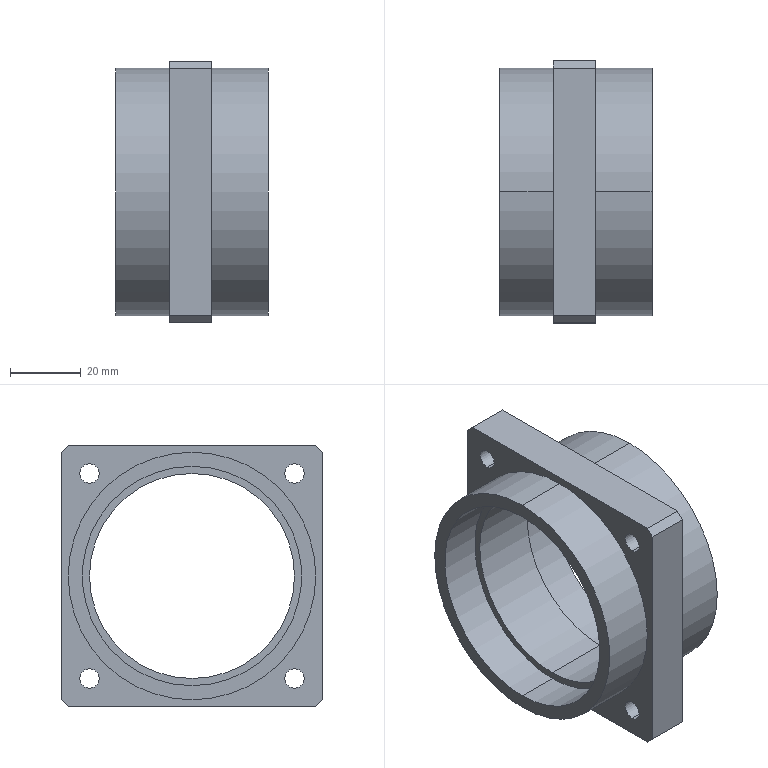Part | STEP file | PN_0025 Bearing Block_Default | 1 solid | 44 faces | box 43 x 74 x 74 mm | volume 59989 mm3 | cylinder 26 | plane 18 | commonest cylinder face diameters 5.5 x8 9.5 x8 62 x4 70 x4 58 x2